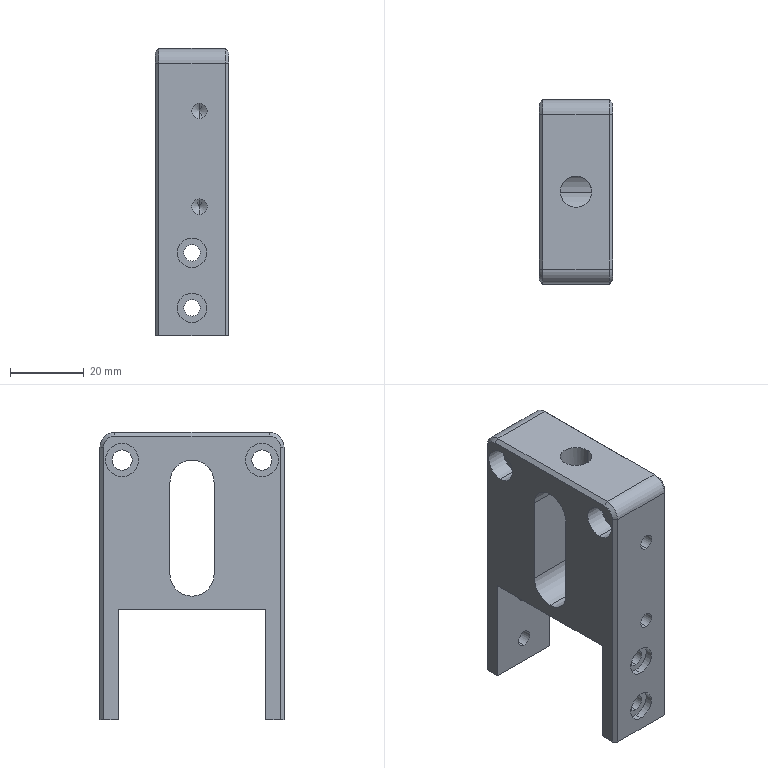Part | STEP file | PN_0011 | 1 solid | 81 faces | box 20 x 50 x 78 mm | volume 41890 mm3 | cylinder 42 | plane 27 | cone 12 | commonest cylinder face diameters 8 x10 4.2 x8 4.5 x8 5.5 x4 9 x4 12 x3